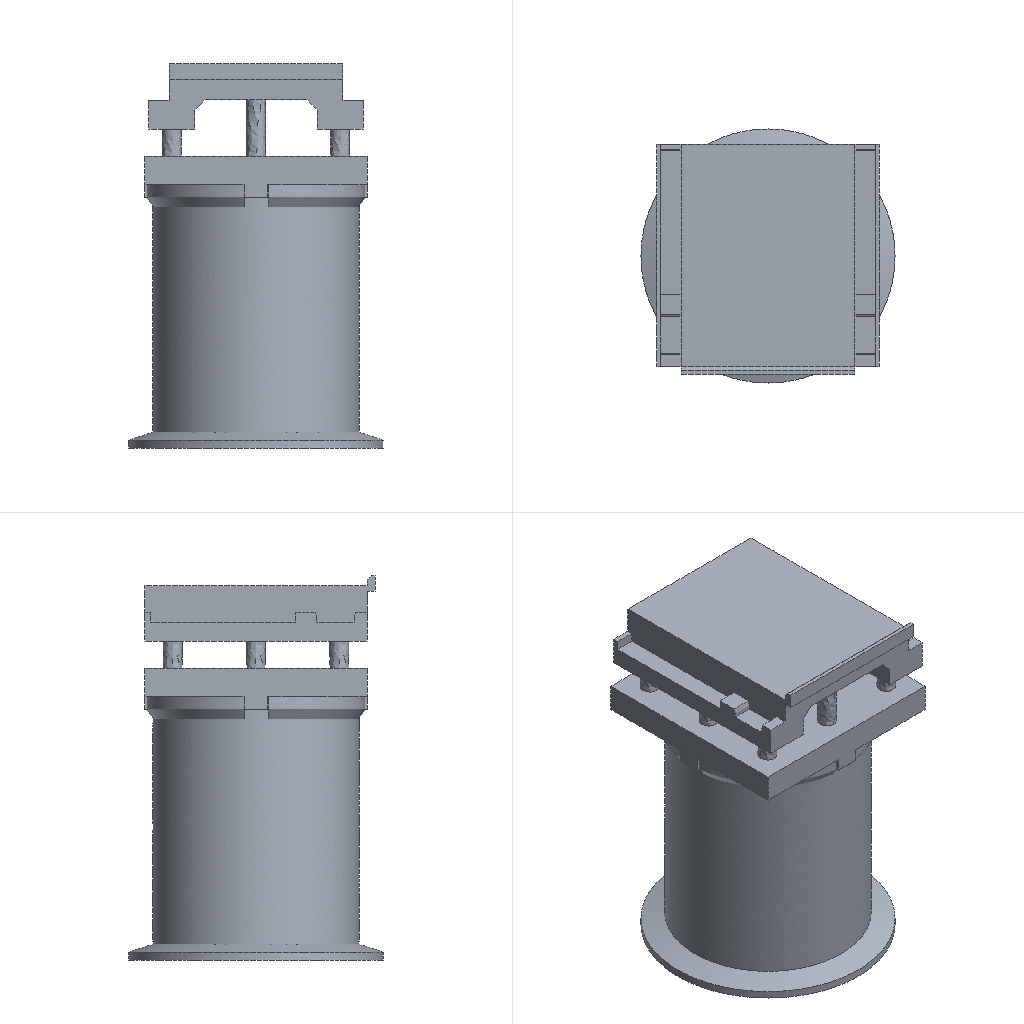Simulation study | ansys workbench
Set-up summary:
category,name,step,type,value,unit,region
solver,ansys_workbench
units,SI m-kg-s (Pa),,stated,"/units,MKS"
analysis,deck-1/LS1,,static
load_step,deck-1/LS1,deck-1/LS1,static,nsubst=1; time=0.01
analysis,deck-2/LS1,,static
load_step,deck-2/LS1,deck-2/LS1,static,nsubst=1; time=1
analysis,deck-3/LS1,,static
load_step,deck-3/LS1,deck-3/LS1,static,nsubst=1; time=1
analysis,deck-4/LS1,,static
load_step,deck-4/LS1,deck-4/LS1,static,nsubst=1; time=1
mesh,deck-1.dat,,nodes,150303
mesh,deck-1.dat,,elements,94954
element_type,SOLID187,,,87505,,deck-1.dat
element_type,SURF154,,,7449,,deck-1.dat
mesh,deck-2.dat,,nodes,150303
mesh,deck-2.dat,,elements,94954
element_type,SOLID187,,,87505,,deck-2.dat
element_type,SURF154,,,7449,,deck-2.dat
mesh,deck-3.dat,,nodes,150303
mesh,deck-3.dat,,elements,94954
element_type,SOLID187,,,87505,,deck-3.dat
element_type,SURF154,,,7449,,deck-3.dat
mesh,deck-4.dat,,nodes,150303
mesh,deck-4.dat,,elements,94954
element_type,SOLID187,,,87505,,deck-4.dat
element_type,SURF154,,,7449,,deck-4.dat
material,Concrete,,E,3e+10,Pa
material,Concrete,,nu,0.18
material,Concrete,,density,2300,kg m^-3
material,Concrete,,conductivity,0.72,W m^-1 C^-1
material,Concrete,,specific_heat,780,J kg^-1 C^-1
material,Concrete,,cte,1.4e-05,C^-1
load,Define Force Using Surface Effect Elements,deck-1/LS1,surface-effect pres face 2,-21371.3,,SURF154 #2
load,ACEL,deck-1/LS1,gravity (ACEL; gravity acts opposite),"9.807 [dir=(0, 0, -1)]",,all
load,Define Force Using Surface Effect Elements,deck-2/LS1,surface-effect pres face 2,-859.904,,SURF154 #2
load,ACEL,deck-2/LS1,gravity (ACEL; gravity acts opposite),"9.807 [dir=(0, 0, -1)]",,all
load,Define Force Using Surface Effect Elements,deck-3/LS1,surface-effect pres face 2,-1170.24,,SURF154 #2
load,ACEL,deck-3/LS1,gravity (ACEL; gravity acts opposite),"9.807 [dir=(0, 0, -1)]",,all
load,Define Force Using Surface Effect Elements,deck-4/LS1,surface-effect pres face 2,-1934.78,,SURF154 #2
load,ACEL,deck-4/LS1,gravity (ACEL; gravity acts opposite),"9.807 [dir=(0, 0, -1)]",,all
bc,Fixed Supports,deck-1/model,fixed,[dofs=ALL],,_FIXEDSU
bc,Fixed Supports,deck-2/model,fixed,[dofs=ALL],,_FIXEDSU
bc,Fixed Supports,deck-3/model,fixed,[dofs=ALL],,_FIXEDSU
bc,Fixed Supports,deck-4/model,fixed,[dofs=ALL],,_FIXEDSU
named_set,_FIXEDSU,,node,7355
named_set,_FIXEDSU,,node,7355
named_set,_FIXEDSU,,node,7355
named_set,_FIXEDSU,,node,7355
Results summary:
result,analyses[0].index,,,1
result,analyses[0].system,,,SYS
result,analyses[0].deck,,,deck-1.dat
result,analyses[0].solve_status,,,completed
result,analyses[0].analysis_type,,,static
result,analyses[0].physics,,,mechanical
result,analyses[0].unit_system,,,"MKS: m, kg, N, s, V, A, degC"
result,analyses[0].n_sets,,,1
result,analyses[0].load_steps[0].set,set=1,,1
result,analyses[0].load_steps[0].time_or_freq,set=1,,0.01
result,analyses[0].load_steps[0].max_displacement_magnitude,set=1,,0.0003597
result,analyses[0].load_steps[0].max_von_mises_nodal,set=1,,1.91301e+06
result,analyses[0].load_steps[0].reaction_force_sum_xyz[1],set=1,,0.001167
result,analyses[0].load_steps[0].reaction_force_sum_xyz[2],set=1,,6.432e+06
result,analyses[0].load_steps[0].reaction_force_sum_xyz[3],set=1,,6.86033e+07
result,analyses[1].index,,,2
result,analyses[1].system,,,SYS-1
result,analyses[1].deck,,,deck-2.dat
result,analyses[1].solve_status,,,completed
result,analyses[1].analysis_type,,,static
result,analyses[1].physics,,,mechanical
result,analyses[1].unit_system,,,"MKS: m, kg, N, s, V, A, degC"
result,analyses[1].n_sets,,,1
result,analyses[1].load_steps[0].set,set=1,,1
result,analyses[1].load_steps[0].time_or_freq,set=1,,1
result,analyses[1].load_steps[0].max_displacement_magnitude,set=1,,0.0003399
result,analyses[1].load_steps[0].max_von_mises_nodal,set=1,,1.73818e+06
result,analyses[1].load_steps[0].reaction_force_sum_xyz[1],set=1,,-0.0004041
result,analyses[1].load_steps[0].reaction_force_sum_xyz[2],set=1,,258800
result,analyses[1].load_steps[0].reaction_force_sum_xyz[3],set=1,,6.86033e+07
result,analyses[2].index,,,3
result,analyses[2].system,,,SYS-2
result,analyses[2].deck,,,deck-3.dat
result,analyses[2].solve_status,,,completed
result,analyses[2].analysis_type,,,static
result,analyses[2].physics,,,mechanical
result,analyses[2].unit_system,,,"MKS: m, kg, N, s, V, A, degC"
result,analyses[2].n_sets,,,1
result,analyses[2].load_steps[0].set,set=1,,1
result,analyses[2].load_steps[0].time_or_freq,set=1,,1
result,analyses[2].load_steps[0].max_displacement_magnitude,set=1,,0.00034
result,analyses[2].load_steps[0].max_von_mises_nodal,set=1,,1.73818e+06
result,analyses[2].load_steps[0].reaction_force_sum_xyz[1],set=1,,-0.0003648
result,analyses[2].load_steps[0].reaction_force_sum_xyz[2],set=1,,352200
result,analyses[2].load_steps[0].reaction_force_sum_xyz[3],set=1,,6.86033e+07
result,analyses[3].index,,,4
result,analyses[3].system,,,SYS-3
result,analyses[3].deck,,,deck-4.dat
result,analyses[3].solve_status,,,completed
result,analyses[3].analysis_type,,,static
result,analyses[3].physics,,,mechanical
result,analyses[3].unit_system,,,"MKS: m, kg, N, s, V, A, degC"
result,analyses[3].n_sets,,,1
result,analyses[3].load_steps[0].set,set=1,,1
result,analyses[3].load_steps[0].time_or_freq,set=1,,1
result,analyses[3].load_steps[0].max_displacement_magnitude,set=1,,0.0003406
result,analyses[3].load_steps[0].max_von_mises_nodal,set=1,,1.73818e+06
result,analyses[3].load_steps[0].reaction_force_sum_xyz[1],set=1,,-0.0003153
result,analyses[3].load_steps[0].reaction_force_sum_xyz[2],set=1,,582300
result,analyses[3].load_steps[0].reaction_force_sum_xyz[3],set=1,,6.86033e+07
result,geometry_export[0][0],,,.step
result,geometry_export[0][1],,,ok
result,geometry_export[0][2],,,1